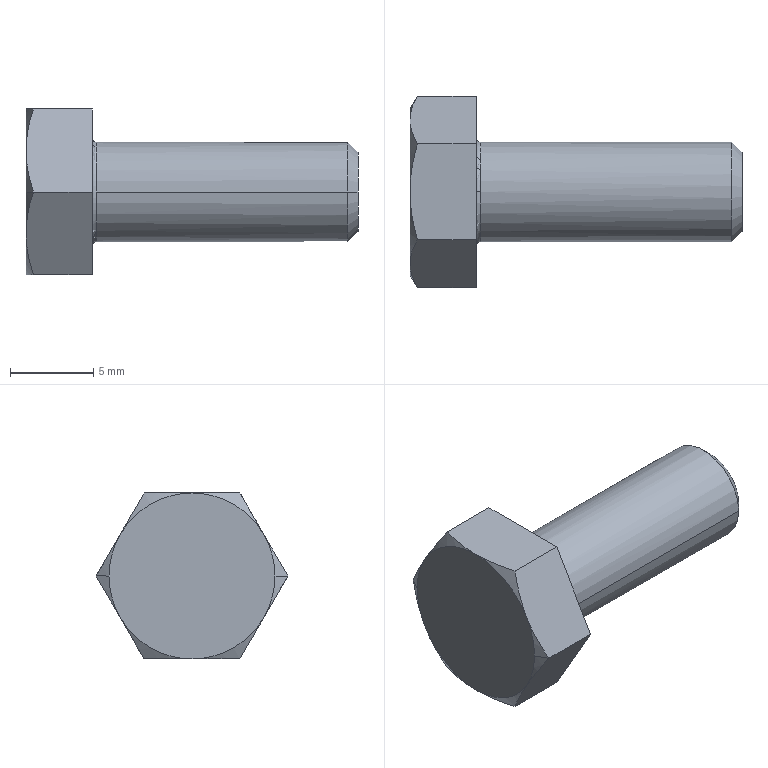Part | STEP file | KS B 1002 - C  M 6 x 16 | 1 solid | 23 faces | box 20 x 11.547 x 10 mm | volume 794.666 mm3 | cone 10 | plane 9 | torus 2 | cylinder 2 | commonest cylinder face diameters 6 x2